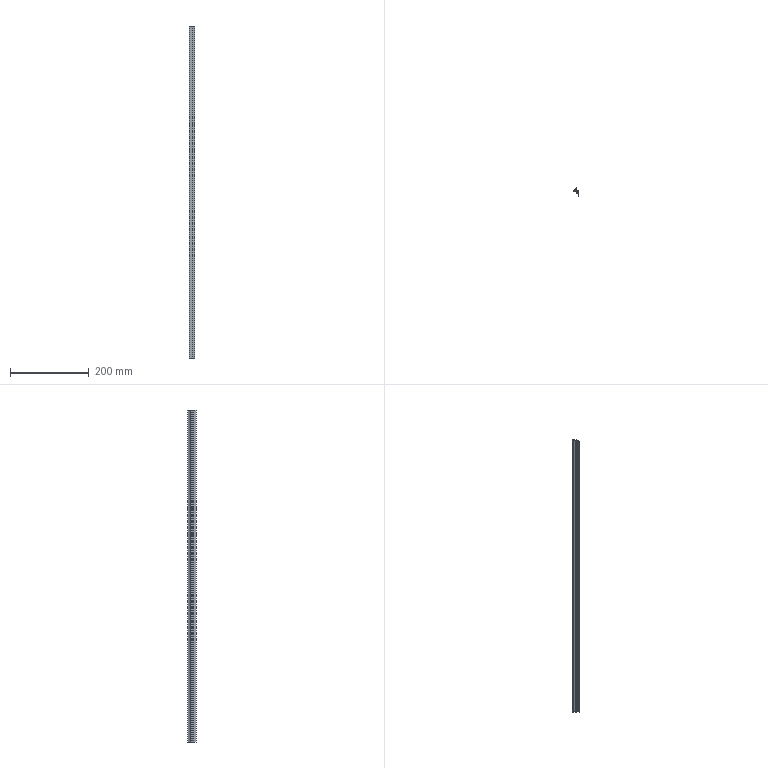Part | SolidWorks | features BaseBody 1, ICE 1, MoveFace 1 | 1 solid | 27 faces | box 14 x 20.3 x 842 mm | volume 42871 mm3 | plane 20 | cylinder 7 | commonest cylinder face diameters 0.387 x2 0.8 x2 0.4 x1 20 x1 22 x1
STEP:
#1=CARTESIAN_POINT('',(-5.304,-0.625,200.));
#2=VERTEX_POINT('',#1);
#3=CARTESIAN_POINT('',(-5.449,-0.8125,200.));
#4=VERTEX_POINT('',#3);
#5=CARTESIAN_POINT('',(-5.255,-0.8125,200.));
#6=DIRECTION('',(0.,0.,1.));
#7=DIRECTION('',(-1.,0.,0.));
#8=AXIS2_PLACEMENT_3D('',#5,#6,#7);
#9=CIRCLE('',#8,0.1937);
#10=EDGE_CURVE('',#2,#4,#9,.T.);
#11=ORIENTED_EDGE('',*,*,#10,.T.);
#12=CARTESIAN_POINT('',(-5.449,-0.8125,-642.));
#13=VERTEX_POINT('',#12);
#14=CARTESIAN_POINT('',(-5.449,-0.8125,230.));
#15=DIRECTION('',(0.,0.,-1.));
#16=VECTOR('',#15,1000.);
#17=LINE('',#14,#16);
#18=EDGE_CURVE('',#4,#13,#17,.T.);
#19=ORIENTED_EDGE('',*,*,#18,.T.);
#20=CARTESIAN_POINT('',(-5.304,-0.625,-642.));
#21=VERTEX_POINT('',#20);
#22=CARTESIAN_POINT('',(-5.255,-0.8125,-642.));
#23=DIRECTION('',(0.,0.,-1.));
#24=DIRECTION('',(1.,0.,0.));
#25=AXIS2_PLACEMENT_3D('',#22,#23,#24);
#26=CIRCLE('',#25,0.1937);
#27=EDGE_CURVE('',#13,#21,#26,.T.);
#28=ORIENTED_EDGE('',*,*,#27,.T.);
#29=CARTESIAN_POINT('',(-5.304,-0.625,230.));
#30=DIRECTION('',(0.,0.,-1.));
#31=VECTOR('',#30,1000.);
#32=LINE('',#29,#31);
#33=EDGE_CURVE('',#2,#21,#32,.T.);
#34=ORIENTED_EDGE('',*,*,#33,.F.);
#35=EDGE_LOOP('',(#11,#19,#28,#34));
#36=FACE_OUTER_BOUND('',#35,.T.);
#37=CARTESIAN_POINT('',(-5.255,-0.8125,230.));
#38=DIRECTION('',(0.,0.,-1.));
#39=DIRECTION('',(-1.,0.,0.));
#40=AXIS2_PLACEMENT_3D('',#37,#38,#39);
#41=CYLINDRICAL_SURFACE('',#40,0.1937);
#42=ADVANCED_FACE('',(#36),#41,.F.);
#43=CARTESIAN_POINT('',(5.,-1.,-642.));
#44=VERTEX_POINT('',#43);
#45=CARTESIAN_POINT('',(5.,-14.3,-642.));
#46=VERTEX_POINT('',#45);
#47=CARTESIAN_POINT('',(5.,29.623,-642.));
#48=DIRECTION('',(0.,-1.,0.));
#49=VECTOR('',#48,1000.);
#50=LINE('',#47,#49);
#51=EDGE_CURVE('',#44,#46,#50,.T.);
#52=ORIENTED_EDGE('',*,*,#51,.F.);
#53=CARTESIAN_POINT('',(5.,-1.,200.));
#54=VERTEX_POINT('',#53);
#55=CARTESIAN_POINT('',(5.,-1.,230.));
#56=DIRECTION('',(0.,0.,-1.));
#57=VECTOR('',#56,1000.);
#58=LINE('',#55,#57);
#59=EDGE_CURVE('',#54,#44,#58,.T.);
#60=ORIENTED_EDGE('',*,*,#59,.F.);
#61=CARTESIAN_POINT('',(5.,-14.3,200.));
#62=VERTEX_POINT('',#61);
#63=CARTESIAN_POINT('',(5.,-14.3,200.));
#64=DIRECTION('',(0.,1.,0.));
#65=VECTOR('',#64,1000.);
#66=LINE('',#63,#65);
#67=EDGE_CURVE('',#62,#54,#66,.T.);
#68=ORIENTED_EDGE('',*,*,#67,.F.);
#69=CARTESIAN_POINT('',(5.,-14.3,230.));
#70=DIRECTION('',(0.,0.,1.));
#71=VECTOR('',#70,1000.);
#72=LINE('',#69,#71);
#73=EDGE_CURVE('',#46,#62,#72,.T.);
#74=ORIENTED_EDGE('',*,*,#73,.F.);
#75=EDGE_LOOP('',(#52,#60,#68,#74));
#76=FACE_OUTER_BOUND('',#75,.T.);
#77=CARTESIAN_POINT('',(5.,-14.3,230.));
#78=DIRECTION('',(-1.,0.,0.));
#79=DIRECTION('',(0.,0.,1.));
#80=AXIS2_PLACEMENT_3D('',#77,#78,#79);
#81=PLANE('',#80);
#82=ADVANCED_FACE('',(#76),#81,.F.);
#83=CARTESIAN_POINT('',(-9.,-2.,-642.));
#84=VERTEX_POINT('',#83);
#85=CARTESIAN_POINT('',(-9.,-2.,200.));
#86=VERTEX_POINT('',#85);
#87=CARTESIAN_POINT('',(-9.,-2.,230.));
#88=DIRECTION('',(0.,0.,1.));
#89=VECTOR('',#88,1000.);
#90=LINE('',#87,#89);
#91=EDGE_CURVE('',#84,#86,#90,.T.);
#92=ORIENTED_EDGE('',*,*,#91,.F.);
#93=CARTESIAN_POINT('',(0.9,-2.,-642.));
#94=VERTEX_POINT('',#93);
#95=CARTESIAN_POINT('',(5.,-2.,-642.));
#96=DIRECTION('',(-1.,0.,0.));
#97=VECTOR('',#96,1000.);
#98=LINE('',#95,#97);
#99=EDGE_CURVE('',#94,#84,#98,.T.);
#100=ORIENTED_EDGE('',*,*,#99,.F.);
#101=CARTESIAN_POINT('',(0.9,-2.,200.));
#102=VERTEX_POINT('',#101);
#103=CARTESIAN_POINT('',(0.9,-2.,230.));
#104=DIRECTION('',(0.,0.,-1.));
#105=VECTOR('',#104,1000.);
#106=LINE('',#103,#105);
#107=EDGE_CURVE('',#102,#94,#106,.T.);
#108=ORIENTED_EDGE('',*,*,#107,.F.);
#109=CARTESIAN_POINT('',(5.,-2.,200.));
#110=DIRECTION('',(1.,0.,0.));
#111=VECTOR('',#110,1000.);
#112=LINE('',#109,#111);
#113=EDGE_CURVE('',#86,#102,#112,.T.);
#114=ORIENTED_EDGE('',*,*,#113,.F.);
#115=EDGE_LOOP('',(#92,#100,#108,#114));
#116=FACE_OUTER_BOUND('',#115,.T.);
#117=CARTESIAN_POINT('',(-9.,-2.,230.));
#118=DIRECTION('',(0.,1.,0.));
#119=DIRECTION('',(0.,0.,1.));
#120=AXIS2_PLACEMENT_3D('',#117,#118,#119);
#121=PLANE('',#120);
#122=ADVANCED_FACE('',(#116),#121,.F.);
#123=CARTESIAN_POINT('',(4.,-6.,200.));
#124=VERTEX_POINT('',#123);
#125=CARTESIAN_POINT('',(4.,-3.,200.));
#126=VERTEX_POINT('',#125);
#127=CARTESIAN_POINT('',(4.,29.623,200.));
#128=DIRECTION('',(0.,1.,0.));
#129=VECTOR('',#128,1000.);
#130=LINE('',#127,#129);
#131=EDGE_CURVE('',#124,#126,#130,.T.);
#132=ORIENTED_EDGE('',*,*,#131,.F.);
#133=CARTESIAN_POINT('',(1.,-6.,200.));
#134=VERTEX_POINT('',#133);
#135=CARTESIAN_POINT('',(5.,-6.,200.));
#136=DIRECTION('',(1.,0.,0.));
#137=VECTOR('',#136,1000.);
#138=LINE('',#135,#137);
#139=EDGE_CURVE('',#134,#124,#138,.T.);
#140=ORIENTED_EDGE('',*,*,#139,.F.);
#141=CARTESIAN_POINT('',(1.,-6.7,200.));
#142=VERTEX_POINT('',#141);
#143=CARTESIAN_POINT('',(1.,-6.,200.));
#144=DIRECTION('',(0.,-1.,0.));
#145=VECTOR('',#144,1000.);
#146=LINE('',#143,#145);
#147=EDGE_CURVE('',#134,#142,#146,.T.);
#148=ORIENTED_EDGE('',*,*,#147,.T.);
#149=CARTESIAN_POINT('',(-1.7,-6.7,200.));
#150=VERTEX_POINT('',#149);
#151=CARTESIAN_POINT('',(5.,-6.7,200.));
#152=DIRECTION('',(1.,0.,0.));
#153=VECTOR('',#152,1000.);
#154=LINE('',#151,#153);
#155=EDGE_CURVE('',#150,#142,#154,.T.);
#156=ORIENTED_EDGE('',*,*,#155,.F.);
#157=CARTESIAN_POINT('',(-1.7,-7.7,200.));
#158=VERTEX_POINT('',#157);
#159=CARTESIAN_POINT('',(-1.7,-6.7,200.));
#160=DIRECTION('',(0.,-1.,0.));
#161=VECTOR('',#160,1000.);
#162=LINE('',#159,#161);
#163=EDGE_CURVE('',#150,#158,#162,.T.);
#164=ORIENTED_EDGE('',*,*,#163,.T.);
#165=CARTESIAN_POINT('',(4.,-7.7,200.));
#166=VERTEX_POINT('',#165);
#167=CARTESIAN_POINT('',(5.,-7.7,200.));
#168=DIRECTION('',(-1.,0.,0.));
#169=VECTOR('',#168,1000.);
#170=LINE('',#167,#169);
#171=EDGE_CURVE('',#166,#158,#170,.T.);
#172=ORIENTED_EDGE('',*,*,#171,.F.);
#173=CARTESIAN_POINT('',(4.,-14.3,200.));
#174=VERTEX_POINT('',#173);
#175=CARTESIAN_POINT('',(4.,29.623,200.));
#176=DIRECTION('',(0.,1.,0.));
#177=VECTOR('',#176,1000.);
#178=LINE('',#175,#177);
#179=EDGE_CURVE('',#174,#166,#178,.T.);
#180=ORIENTED_EDGE('',*,*,#179,.F.);
#181=CARTESIAN_POINT('',(5.,-14.3,200.));
#182=DIRECTION('',(-1.,0.,0.));
#183=VECTOR('',#182,1000.);
#184=LINE('',#181,#183);
#185=EDGE_CURVE('',#62,#174,#184,.T.);
#186=ORIENTED_EDGE('',*,*,#185,.F.);
#187=ORIENTED_EDGE('',*,*,#67,.T.);
#188=CARTESIAN_POINT('',(-5.207,-1.,200.));
#189=VERTEX_POINT('',#188);
#190=CARTESIAN_POINT('',(5.,-1.,200.));
#191=DIRECTION('',(1.,0.,0.));
#192=VECTOR('',#191,1000.);
#193=LINE('',#190,#192);
#194=EDGE_CURVE('',#189,#54,#193,.T.);
#195=ORIENTED_EDGE('',*,*,#194,.F.);
#196=CARTESIAN_POINT('',(-5.255,-0.8125,200.));
#197=DIRECTION('',(0.,0.,1.));
#198=DIRECTION('',(-1.,0.,0.));
#199=AXIS2_PLACEMENT_3D('',#196,#197,#198);
#200=CIRCLE('',#199,0.1937);
#201=EDGE_CURVE('',#4,#189,#200,.T.);
#202=ORIENTED_EDGE('',*,*,#201,.F.);
#203=ORIENTED_EDGE('',*,*,#10,.F.);
#204=CARTESIAN_POINT('',(-1.368,3.063,200.));
#205=VERTEX_POINT('',#204);
#206=CARTESIAN_POINT('',(-10.628,9.,200.));
#207=DIRECTION('',(0.,0.,1.));
#208=DIRECTION('',(-1.,0.,0.));
#209=AXIS2_PLACEMENT_3D('',#206,#207,#208);
#210=CIRCLE('',#209,11.);
#211=EDGE_CURVE('',#2,#205,#210,.T.);
#212=ORIENTED_EDGE('',*,*,#211,.T.);
#213=CARTESIAN_POINT('',(-1.,2.955,200.));
#214=VERTEX_POINT('',#213);
#215=CARTESIAN_POINT('',(-1.2,2.955,200.));
#216=DIRECTION('',(0.,0.,1.));
#217=DIRECTION('',(-1.,0.,0.));
#218=AXIS2_PLACEMENT_3D('',#215,#216,#217);
#219=CIRCLE('',#218,0.2);
#220=EDGE_CURVE('',#214,#205,#219,.T.);
#221=ORIENTED_EDGE('',*,*,#220,.F.);
#222=CARTESIAN_POINT('',(-1.,1.5,200.));
#223=VERTEX_POINT('',#222);
#224=CARTESIAN_POINT('',(-1.,2.955,200.));
#225=DIRECTION('',(0.,1.,0.));
#226=VECTOR('',#225,1000.);
#227=LINE('',#224,#226);
#228=EDGE_CURVE('',#223,#214,#227,.T.);
#229=ORIENTED_EDGE('',*,*,#228,.F.);
#230=CARTESIAN_POINT('',(0.,1.5,200.));
#231=VERTEX_POINT('',#230);
#232=CARTESIAN_POINT('',(-1.,1.5,200.));
#233=DIRECTION('',(-1.,0.,0.));
#234=VECTOR('',#233,1000.);
#235=LINE('',#232,#234);
#236=EDGE_CURVE('',#231,#223,#235,.T.);
#237=ORIENTED_EDGE('',*,*,#236,.F.);
#238=CARTESIAN_POINT('',(0.,6.,200.));
#239=VERTEX_POINT('',#238);
#240=CARTESIAN_POINT('',(0.,1.5,200.));
#241=DIRECTION('',(0.,-1.,0.));
#242=VECTOR('',#241,1000.);
#243=LINE('',#240,#242);
#244=EDGE_CURVE('',#239,#231,#243,.T.);
#245=ORIENTED_EDGE('',*,*,#244,.F.);
#246=CARTESIAN_POINT('',(-0.8,6.,200.));
#247=VERTEX_POINT('',#246);
#248=CARTESIAN_POINT('',(0.,6.,200.));
#249=DIRECTION('',(1.,0.,0.));
#250=VECTOR('',#249,1000.);
#251=LINE('',#248,#250);
#252=EDGE_CURVE('',#247,#239,#251,.T.);
#253=ORIENTED_EDGE('',*,*,#252,.F.);
#254=CARTESIAN_POINT('',(-1.178,5.731,200.));
#255=VERTEX_POINT('',#254);
#256=CARTESIAN_POINT('',(-0.8,5.6,200.));
#257=DIRECTION('',(0.,0.,1.));
#258=DIRECTION('',(-1.,0.,0.));
#259=AXIS2_PLACEMENT_3D('',#256,#257,#258);
#260=CIRCLE('',#259,0.4);
#261=EDGE_CURVE('',#247,#255,#260,.T.);
#262=ORIENTED_EDGE('',*,*,#261,.T.);
#263=CARTESIAN_POINT('',(-8.678,-0.8077,200.));
#264=VERTEX_POINT('',#263);
#265=CARTESIAN_POINT('',(-10.628,9.,200.));
#266=DIRECTION('',(0.,0.,1.));
#267=DIRECTION('',(-1.,0.,0.));
#268=AXIS2_PLACEMENT_3D('',#265,#266,#267);
#269=CIRCLE('',#268,10.);
#270=EDGE_CURVE('',#264,#255,#269,.T.);
#271=ORIENTED_EDGE('',*,*,#270,.F.);
#272=CARTESIAN_POINT('',(-9.,-1.2,200.));
#273=VERTEX_POINT('',#272);
#274=CARTESIAN_POINT('',(-8.6,-1.2,200.));
#275=DIRECTION('',(0.,0.,1.));
#276=DIRECTION('',(-1.,0.,0.));
#277=AXIS2_PLACEMENT_3D('',#274,#275,#276);
#278=CIRCLE('',#277,0.4);
#279=EDGE_CURVE('',#264,#273,#278,.T.);
#280=ORIENTED_EDGE('',*,*,#279,.T.);
#281=CARTESIAN_POINT('',(-9.,8.,200.));
#282=DIRECTION('',(0.,-1.,0.));
#283=VECTOR('',#282,1000.);
#284=LINE('',#281,#283);
#285=EDGE_CURVE('',#273,#86,#284,.T.);
#286=ORIENTED_EDGE('',*,*,#285,.T.);
#287=ORIENTED_EDGE('',*,*,#113,.T.);
#288=CARTESIAN_POINT('',(0.9,-3.,200.));
#289=VERTEX_POINT('',#288);
#290=CARTESIAN_POINT('',(0.9,29.623,200.));
#291=DIRECTION('',(0.,1.,0.));
#292=VECTOR('',#291,1000.);
#293=LINE('',#290,#292);
#294=EDGE_CURVE('',#289,#102,#293,.T.);
#295=ORIENTED_EDGE('',*,*,#294,.F.);
#296=CARTESIAN_POINT('',(5.,-3.,200.));
#297=DIRECTION('',(-1.,0.,0.));
#298=VECTOR('',#297,1000.);
#299=LINE('',#296,#298);
#300=EDGE_CURVE('',#126,#289,#299,.T.);
#301=ORIENTED_EDGE('',*,*,#300,.F.);
#302=EDGE_LOOP('',(#132,#140,#148,#156,#164,#172,#180,#186,#187,#195,#202,#203,#212,#221,#229,#237,#245,#253,#262,#271,#280,#286,#287,#295,#301));
#303=FACE_OUTER_BOUND('',#302,.T.);
#304=CARTESIAN_POINT('',(5.,29.623,200.));
#305=DIRECTION('',(0.,0.,-1.));
#306=DIRECTION('',(-1.,0.,0.));
#307=AXIS2_PLACEMENT_3D('',#304,#305,#306);
#308=PLANE('',#307);
#309=ADVANCED_FACE('',(#303),#308,.F.);
#310=ORIENTED_EDGE('',*,*,#185,.T.);
#311=CARTESIAN_POINT('',(4.,-14.3,-642.));
#312=VERTEX_POINT('',#311);
#313=CARTESIAN_POINT('',(4.,-14.3,230.));
#314=DIRECTION('',(0.,0.,1.));
#315=VECTOR('',#314,1000.);
#316=LINE('',#313,#315);
#317=EDGE_CURVE('',#312,#174,#316,.T.);
#318=ORIENTED_EDGE('',*,*,#317,.F.);
#319=CARTESIAN_POINT('',(5.,-14.3,-642.));
#320=DIRECTION('',(-1.,0.,0.));
#321=VECTOR('',#320,1000.);
#322=LINE('',#319,#321);
#323=EDGE_CURVE('',#46,#312,#322,.T.);
#324=ORIENTED_EDGE('',*,*,#323,.F.);
#325=ORIENTED_EDGE('',*,*,#73,.T.);
#326=EDGE_LOOP('',(#310,#318,#324,#325));
#327=FACE_OUTER_BOUND('',#326,.T.);
#328=CARTESIAN_POINT('',(4.,-14.3,230.));
#329=DIRECTION('',(0.,1.,0.));
#330=DIRECTION('',(0.,0.,1.));
#331=AXIS2_PLACEMENT_3D('',#328,#329,#330);
#332=PLANE('',#331);
#333=ADVANCED_FACE('',(#327),#332,.F.);
#334=ORIENTED_EDGE('',*,*,#51,.T.);
#335=ORIENTED_EDGE('',*,*,#323,.T.);
#336=CARTESIAN_POINT('',(4.,-7.7,-642.));
#337=VERTEX_POINT('',#336);
#338=CARTESIAN_POINT('',(4.,-7.7,-642.));
#339=DIRECTION('',(0.,-1.,0.));
#340=VECTOR('',#339,1000.);
#341=LINE('',#338,#340);
#342=EDGE_CURVE('',#337,#312,#341,.T.);
#343=ORIENTED_EDGE('',*,*,#342,.F.);
#344=CARTESIAN_POINT('',(-1.7,-7.7,-642.));
#345=VERTEX_POINT('',#344);
#346=CARTESIAN_POINT('',(-1.7,-7.7,-642.));
#347=DIRECTION('',(1.,0.,0.));
#348=VECTOR('',#347,1000.);
#349=LINE('',#346,#348);
#350=EDGE_CURVE('',#345,#337,#349,.T.);
#351=ORIENTED_EDGE('',*,*,#350,.F.);
#352=CARTESIAN_POINT('',(-1.7,-6.7,-642.));
#353=VERTEX_POINT('',#352);
#354=CARTESIAN_POINT('',(-1.7,29.623,-642.));
#355=DIRECTION('',(0.,1.,0.));
#356=VECTOR('',#355,1000.);
#357=LINE('',#354,#356);
#358=EDGE_CURVE('',#345,#353,#357,.T.);
#359=ORIENTED_EDGE('',*,*,#358,.T.);
#360=CARTESIAN_POINT('',(1.,-6.7,-642.));
#361=VERTEX_POINT('',#360);
#362=CARTESIAN_POINT('',(1.,-6.7,-642.));
#363=DIRECTION('',(-1.,0.,0.));
#364=VECTOR('',#363,1000.);
#365=LINE('',#362,#364);
#366=EDGE_CURVE('',#361,#353,#365,.T.);
#367=ORIENTED_EDGE('',*,*,#366,.F.);
#368=CARTESIAN_POINT('',(1.,-6.,-642.));
#369=VERTEX_POINT('',#368);
#370=CARTESIAN_POINT('',(1.,29.623,-642.));
#371=DIRECTION('',(0.,1.,0.));
#372=VECTOR('',#371,1000.);
#373=LINE('',#370,#372);
#374=EDGE_CURVE('',#361,#369,#373,.T.);
#375=ORIENTED_EDGE('',*,*,#374,.T.);
#376=CARTESIAN_POINT('',(4.,-6.,-642.));
#377=VERTEX_POINT('',#376);
#378=CARTESIAN_POINT('',(4.,-6.,-642.));
#379=DIRECTION('',(-1.,0.,0.));
#380=VECTOR('',#379,1000.);
#381=LINE('',#378,#380);
#382=EDGE_CURVE('',#377,#369,#381,.T.);
#383=ORIENTED_EDGE('',*,*,#382,.F.);
#384=CARTESIAN_POINT('',(4.,-3.,-642.));
#385=VERTEX_POINT('',#384);
#386=CARTESIAN_POINT('',(4.,-3.,-642.));
#387=DIRECTION('',(0.,-1.,0.));
#388=VECTOR('',#387,1000.);
#389=LINE('',#386,#388);
#390=EDGE_CURVE('',#385,#377,#389,.T.);
#391=ORIENTED_EDGE('',*,*,#390,.F.);
#392=CARTESIAN_POINT('',(0.9,-3.,-642.));
#393=VERTEX_POINT('',#392);
#394=CARTESIAN_POINT('',(0.9,-3.,-642.));
#395=DIRECTION('',(1.,0.,0.));
#396=VECTOR('',#395,1000.);
#397=LINE('',#394,#396);
#398=EDGE_CURVE('',#393,#385,#397,.T.);
#399=ORIENTED_EDGE('',*,*,#398,.F.);
#400=CARTESIAN_POINT('',(0.9,-2.,-642.));
#401=DIRECTION('',(0.,-1.,0.));
#402=VECTOR('',#401,1000.);
#403=LINE('',#400,#402);
#404=EDGE_CURVE('',#94,#393,#403,.T.);
#405=ORIENTED_EDGE('',*,*,#404,.F.);
#406=ORIENTED_EDGE('',*,*,#99,.T.);
#407=CARTESIAN_POINT('',(-9.,-1.2,-642.));
#408=VERTEX_POINT('',#407);
#409=CARTESIAN_POINT('',(-9.,-1.2,-642.));
#410=DIRECTION('',(0.,-1.,0.));
#411=VECTOR('',#410,1000.);
#412=LINE('',#409,#411);
#413=EDGE_CURVE('',#408,#84,#412,.T.);
#414=ORIENTED_EDGE('',*,*,#413,.F.);
#415=CARTESIAN_POINT('',(-8.678,-0.8077,-642.));
#416=VERTEX_POINT('',#415);
#417=CARTESIAN_POINT('',(-8.6,-1.2,-642.));
#418=DIRECTION('',(0.,0.,-1.));
#419=DIRECTION('',(1.,0.,0.));
#420=AXIS2_PLACEMENT_3D('',#417,#418,#419);
#421=CIRCLE('',#420,0.4);
#422=EDGE_CURVE('',#408,#416,#421,.T.);
#423=ORIENTED_EDGE('',*,*,#422,.T.);
#424=CARTESIAN_POINT('',(-1.178,5.731,-642.));
#425=VERTEX_POINT('',#424);
#426=CARTESIAN_POINT('',(-10.628,9.,-642.));
#427=DIRECTION('',(0.,0.,-1.));
#428=DIRECTION('',(1.,0.,0.));
#429=AXIS2_PLACEMENT_3D('',#426,#427,#428);
#430=CIRCLE('',#429,10.);
#431=EDGE_CURVE('',#425,#416,#430,.T.);
#432=ORIENTED_EDGE('',*,*,#431,.F.);
#433=CARTESIAN_POINT('',(-0.8,6.,-642.));
#434=VERTEX_POINT('',#433);
#435=CARTESIAN_POINT('',(-0.8,5.6,-642.));
#436=DIRECTION('',(0.,0.,-1.));
#437=DIRECTION('',(1.,0.,0.));
#438=AXIS2_PLACEMENT_3D('',#435,#436,#437);
#439=CIRCLE('',#438,0.4);
#440=EDGE_CURVE('',#425,#434,#439,.T.);
#441=ORIENTED_EDGE('',*,*,#440,.T.);
#442=CARTESIAN_POINT('',(0.,6.,-642.));
#443=VERTEX_POINT('',#442);
#444=CARTESIAN_POINT('',(0.,6.,-642.));
#445=DIRECTION('',(-1.,0.,0.));
#446=VECTOR('',#445,1000.);
#447=LINE('',#444,#446);
#448=EDGE_CURVE('',#443,#434,#447,.T.);
#449=ORIENTED_EDGE('',*,*,#448,.F.);
#450=CARTESIAN_POINT('',(0.,1.5,-642.));
#451=VERTEX_POINT('',#450);
#452=CARTESIAN_POINT('',(0.,1.5,-642.));
#453=DIRECTION('',(0.,1.,0.));
#454=VECTOR('',#453,1000.);
#455=LINE('',#452,#454);
#456=EDGE_CURVE('',#451,#443,#455,.T.);
#457=ORIENTED_EDGE('',*,*,#456,.F.);
#458=CARTESIAN_POINT('',(-1.,1.5,-642.));
#459=VERTEX_POINT('',#458);
#460=CARTESIAN_POINT('',(-1.,1.5,-642.));
#461=DIRECTION('',(1.,0.,0.));
#462=VECTOR('',#461,1000.);
#463=LINE('',#460,#462);
#464=EDGE_CURVE('',#459,#451,#463,.T.);
#465=ORIENTED_EDGE('',*,*,#464,.F.);
#466=CARTESIAN_POINT('',(-1.,2.955,-642.));
#467=VERTEX_POINT('',#466);
#468=CARTESIAN_POINT('',(-1.,2.955,-642.));
#469=DIRECTION('',(0.,-1.,0.));
#470=VECTOR('',#469,1000.);
#471=LINE('',#468,#470);
#472=EDGE_CURVE('',#467,#459,#471,.T.);
#473=ORIENTED_EDGE('',*,*,#472,.F.);
#474=CARTESIAN_POINT('',(-1.368,3.063,-642.));
#475=VERTEX_POINT('',#474);
#476=CARTESIAN_POINT('',(-1.2,2.955,-642.));
#477=DIRECTION('',(0.,0.,-1.));
#478=DIRECTION('',(1.,0.,0.));
#479=AXIS2_PLACEMENT_3D('',#476,#477,#478);
#480=CIRCLE('',#479,0.2);
#481=EDGE_CURVE('',#475,#467,#480,.T.);
#482=ORIENTED_EDGE('',*,*,#481,.F.);
#483=CARTESIAN_POINT('',(-10.628,9.,-642.));
#484=DIRECTION('',(0.,0.,-1.));
#485=DIRECTION('',(1.,0.,0.));
#486=AXIS2_PLACEMENT_3D('',#483,#484,#485);
#487=CIRCLE('',#486,11.);
#488=EDGE_CURVE('',#475,#21,#487,.T.);
#489=ORIENTED_EDGE('',*,*,#488,.T.);
#490=ORIENTED_EDGE('',*,*,#27,.F.);
#491=CARTESIAN_POINT('',(-5.207,-1.,-642.));
#492=VERTEX_POINT('',#491);
#493=CARTESIAN_POINT('',(-5.255,-0.8125,-642.));
#494=DIRECTION('',(0.,0.,-1.));
#495=DIRECTION('',(1.,0.,0.));
#496=AXIS2_PLACEMENT_3D('',#493,#494,#495);
#497=CIRCLE('',#496,0.1937);
#498=EDGE_CURVE('',#492,#13,#497,.T.);
#499=ORIENTED_EDGE('',*,*,#498,.F.);
#500=CARTESIAN_POINT('',(5.,-1.,-642.));
#501=DIRECTION('',(-1.,0.,0.));
#502=VECTOR('',#501,1000.);
#503=LINE('',#500,#502);
#504=EDGE_CURVE('',#44,#492,#503,.T.);
#505=ORIENTED_EDGE('',*,*,#504,.F.);
#506=EDGE_LOOP('',(#334,#335,#343,#351,#359,#367,#375,#383,#391,#399,#405,#406,#414,#423,#432,#441,#449,#457,#465,#473,#482,#489,#490,#499,#505));
#507=FACE_OUTER_BOUND('',#506,.T.);
#508=CARTESIAN_POINT('',(5.,29.623,-642.));
#509=DIRECTION('',(0.,0.,1.));
#510=DIRECTION('',(1.,0.,0.));
#511=AXIS2_PLACEMENT_3D('',#508,#509,#510);
#512=PLANE('',#511);
#513=ADVANCED_FACE('',(#507),#512,.F.);
#514=ORIENTED_EDGE('',*,*,#59,.T.);
#515=ORIENTED_EDGE('',*,*,#504,.T.);
#516=CARTESIAN_POINT('',(-5.207,-1.,230.));
#517=DIRECTION('',(0.,0.,-1.));
#518=VECTOR('',#517,1000.);
#519=LINE('',#516,#518);
#520=EDGE_CURVE('',#189,#492,#519,.T.);
#521=ORIENTED_EDGE('',*,*,#520,.F.);
#522=ORIENTED_EDGE('',*,*,#194,.T.);
#523=EDGE_LOOP('',(#514,#515,#521,#522));
#524=FACE_OUTER_BOUND('',#523,.T.);
#525=CARTESIAN_POINT('',(5.,-1.,230.));
#526=DIRECTION('',(0.,-1.,0.));
#527=DIRECTION('',(0.,0.,-1.));
#528=AXIS2_PLACEMENT_3D('',#525,#526,#527);
#529=PLANE('',#528);
#530=ADVANCED_FACE('',(#524),#529,.F.);
#531=CARTESIAN_POINT('',(-9.,-1.2,230.));
#532=DIRECTION('',(0.,0.,1.));
#533=VECTOR('',#532,1000.);
#534=LINE('',#531,#533);
#535=EDGE_CURVE('',#408,#273,#534,.T.);
#536=ORIENTED_EDGE('',*,*,#535,.F.);
#537=ORIENTED_EDGE('',*,*,#413,.T.);
#538=ORIENTED_EDGE('',*,*,#91,.T.);
#539=ORIENTED_EDGE('',*,*,#285,.F.);
#540=EDGE_LOOP('',(#536,#537,#538,#539));
#541=FACE_OUTER_BOUND('',#540,.T.);
#542=CARTESIAN_POINT('',(-9.,-1.2,230.));
#543=DIRECTION('',(1.,0.,0.));
#544=DIRECTION('',(0.,0.,-1.));
#545=AXIS2_PLACEMENT_3D('',#542,#543,#544);
#546=PLANE('',#545);
#547=ADVANCED_FACE('',(#541),#546,.F.);
#548=ORIENTED_EDGE('',*,*,#294,.T.);
#549=ORIENTED_EDGE('',*,*,#107,.T.);
#550=ORIENTED_EDGE('',*,*,#404,.T.);
#551=CARTESIAN_POINT('',(0.9,-3.,230.));
#552=DIRECTION('',(0.,0.,-1.));
#553=VECTOR('',#552,1000.);
#554=LINE('',#551,#553);
#555=EDGE_CURVE('',#289,#393,#554,.T.);
#556=ORIENTED_EDGE('',*,*,#555,.F.);
#557=EDGE_LOOP('',(#548,#549,#550,#556));
#558=FACE_OUTER_BOUND('',#557,.T.);
#559=CARTESIAN_POINT('',(0.9,-2.,230.));
#560=DIRECTION('',(1.,0.,0.));
#561=DIRECTION('',(0.,0.,-1.));
#562=AXIS2_PLACEMENT_3D('',#559,#560,#561);
#563=PLANE('',#562);
#564=ADVANCED_FACE('',(#558),#563,.F.);
#565=ORIENTED_EDGE('',*,*,#300,.T.);
#566=ORIENTED_EDGE('',*,*,#555,.T.);
#567=ORIENTED_EDGE('',*,*,#398,.T.);
#568=CARTESIAN_POINT('',(4.,-3.,230.));
#569=DIRECTION('',(0.,0.,-1.));
#570=VECTOR('',#569,1000.);
#571=LINE('',#568,#570);
#572=EDGE_CURVE('',#126,#385,#571,.T.);
#573=ORIENTED_EDGE('',*,*,#572,.F.);
#574=EDGE_LOOP('',(#565,#566,#567,#573));
#575=FACE_OUTER_BOUND('',#574,.T.);
#576=CARTESIAN_POINT('',(0.9,-3.,230.));
#577=DIRECTION('',(0.,1.,0.));
#578=DIRECTION('',(0.,0.,1.));
#579=AXIS2_PLACEMENT_3D('',#576,#577,#578);
#580=PLANE('',#579);
#581=ADVANCED_FACE('',(#575),#580,.F.);
#582=ORIENTED_EDGE('',*,*,#131,.T.);
#583=ORIENTED_EDGE('',*,*,#572,.T.);
#584=ORIENTED_EDGE('',*,*,#390,.T.);
#585=CARTESIAN_POINT('',(4.,-6.,230.));
#586=DIRECTION('',(0.,0.,-1.));
#587=VECTOR('',#586,1000.);
#588=LINE('',#585,#587);
#589=EDGE_CURVE('',#124,#377,#588,.T.);
#590=ORIENTED_EDGE('',*,*,#589,.F.);
#591=EDGE_LOOP('',(#582,#583,#584,#590));
#592=FACE_OUTER_BOUND('',#591,.T.);
#593=CARTESIAN_POINT('',(4.,-3.,230.));
#594=DIRECTION('',(1.,0.,0.));
#595=DIRECTION('',(0.,0.,-1.));
#596=AXIS2_PLACEMENT_3D('',#593,#594,#595);
#597=PLANE('',#596);
#598=ADVANCED_FACE('',(#592),#597,.F.);
#599=ORIENTED_EDGE('',*,*,#139,.T.);
#600=ORIENTED_EDGE('',*,*,#589,.T.);
#601=ORIENTED_EDGE('',*,*,#382,.T.);
#602=CARTESIAN_POINT('',(1.,-6.,230.));
#603=DIRECTION('',(0.,0.,-1.));
#604=VECTOR('',#603,1000.);
#605=LINE('',#602,#604);
#606=EDGE_CURVE('',#134,#369,#605,.T.);
#607=ORIENTED_EDGE('',*,*,#606,.F.);
#608=EDGE_LOOP('',(#599,#600,#601,#607));
#609=FACE_OUTER_BOUND('',#608,.T.);
#610=CARTESIAN_POINT('',(4.,-6.,230.));
#611=DIRECTION('',(0.,-1.,0.));
#612=DIRECTION('',(0.,0.,-1.));
#613=AXIS2_PLACEMENT_3D('',#610,#611,#612);
#614=PLANE('',#613);
#615=ADVANCED_FACE('',(#609),#614,.F.);
#616=ORIENTED_EDGE('',*,*,#155,.T.);
#617=CARTESIAN_POINT('',(1.,-6.7,230.));
#618=DIRECTION('',(0.,0.,1.));
#619=VECTOR('',#618,1000.);
#620=LINE('',#617,#619);
#621=EDGE_CURVE('',#361,#142,#620,.T.);
#622=ORIENTED_EDGE('',*,*,#621,.F.);
#623=ORIENTED_EDGE('',*,*,#366,.T.);
#624=CARTESIAN_POINT('',(-1.7,-6.7,230.));
#625=DIRECTION('',(0.,0.,-1.));
#626=VECTOR('',#625,1000.);
#627=LINE('',#624,#626);
#628=EDGE_CURVE('',#150,#353,#627,.T.);
#629=ORIENTED_EDGE('',*,*,#628,.F.);
#630=EDGE_LOOP('',(#616,#622,#623,#629));
#631=FACE_OUTER_BOUND('',#630,.T.);
#632=CARTESIAN_POINT('',(1.,-6.7,230.));
#633=DIRECTION('',(0.,-1.,0.));
#634=DIRECTION('',(0.,0.,-1.));
#635=AXIS2_PLACEMENT_3D('',#632,#633,#634);
#636=PLANE('',#635);
#637=ADVANCED_FACE('',(#631),#636,.F.);
#638=ORIENTED_EDGE('',*,*,#171,.T.);
#639=CARTESIAN_POINT('',(-1.7,-7.7,230.));
#640=DIRECTION('',(0.,0.,1.));
#641=VECTOR('',#640,1000.);
#642=LINE('',#639,#641);
#643=EDGE_CURVE('',#345,#158,#642,.T.);
#644=ORIENTED_EDGE('',*,*,#643,.F.);
#645=ORIENTED_EDGE('',*,*,#350,.T.);
#646=CARTESIAN_POINT('',(4.,-7.7,230.));
#647=DIRECTION('',(0.,0.,-1.));
#648=VECTOR('',#647,1000.);
#649=LINE('',#646,#648);
#650=EDGE_CURVE('',#166,#337,#649,.T.);
#651=ORIENTED_EDGE('',*,*,#650,.F.);
#652=EDGE_LOOP('',(#638,#644,#645,#651));
#653=FACE_OUTER_BOUND('',#652,.T.);
#654=CARTESIAN_POINT('',(-1.7,-7.7,230.));
#655=DIRECTION('',(0.,1.,0.));
#656=DIRECTION('',(0.,0.,1.));
#657=AXIS2_PLACEMENT_3D('',#654,#655,#656);
#658=PLANE('',#657);
#659=ADVANCED_FACE('',(#653),#658,.F.);
#660=ORIENTED_EDGE('',*,*,#179,.T.);
#661=ORIENTED_EDGE('',*,*,#650,.T.);
#662=ORIENTED_EDGE('',*,*,#342,.T.);
#663=ORIENTED_EDGE('',*,*,#317,.T.);
#664=EDGE_LOOP('',(#660,#661,#662,#663));
#665=FACE_OUTER_BOUND('',#664,.T.);
#666=CARTESIAN_POINT('',(4.,-7.7,230.));
#667=DIRECTION('',(1.,0.,0.));
#668=DIRECTION('',(0.,0.,-1.));
#669=AXIS2_PLACEMENT_3D('',#666,#667,#668);
#670=PLANE('',#669);
#671=ADVANCED_FACE('',(#665),#670,.F.);
#672=ORIENTED_EDGE('',*,*,#18,.F.);
#673=ORIENTED_EDGE('',*,*,#201,.T.);
#674=ORIENTED_EDGE('',*,*,#520,.T.);
#675=ORIENTED_EDGE('',*,*,#498,.T.);
#676=EDGE_LOOP('',(#672,#673,#674,#675));
#677=FACE_OUTER_BOUND('',#676,.T.);
#678=CARTESIAN_POINT('',(-5.255,-0.8125,230.));
#679=DIRECTION('',(0.,0.,-1.));
#680=DIRECTION('',(-1.,0.,0.));
#681=AXIS2_PLACEMENT_3D('',#678,#679,#680);
#682=CYLINDRICAL_SURFACE('',#681,0.1937);
#683=ADVANCED_FACE('',(#677),#682,.F.);
#684=CARTESIAN_POINT('',(-1.,2.955,230.));
#685=DIRECTION('',(0.,0.,1.));
#686=VECTOR('',#685,1000.);
#687=LINE('',#684,#686);
#688=EDGE_CURVE('',#467,#214,#687,.T.);
#689=ORIENTED_EDGE('',*,*,#688,.F.);
#690=ORIENTED_EDGE('',*,*,#472,.T.);
#691=CARTESIAN_POINT('',(-1.,1.5,230.));
#692=DIRECTION('',(0.,0.,-1.));
#693=VECTOR('',#692,1000.);
#694=LINE('',#691,#693);
#695=EDGE_CURVE('',#223,#459,#694,.T.);
#696=ORIENTED_EDGE('',*,*,#695,.F.);
#697=ORIENTED_EDGE('',*,*,#228,.T.);
#698=EDGE_LOOP('',(#689,#690,#696,#697));
#699=FACE_OUTER_BOUND('',#698,.T.);
#700=CARTESIAN_POINT('',(-1.,2.955,230.));
#701=DIRECTION('',(1.,0.,0.));
#702=DIRECTION('',(0.,0.,-1.));
#703=AXIS2_PLACEMENT_3D('',#700,#701,#702);
#704=PLANE('',#703);
#705=ADVANCED_FACE('',(#699),#704,.F.);
#706=ORIENTED_EDGE('',*,*,#488,.F.);
#707=CARTESIAN_POINT('',(-1.368,3.063,230.));
#708=DIRECTION('',(0.,0.,1.));
#709=VECTOR('',#708,1000.);
#710=LINE('',#707,#709);
#711=EDGE_CURVE('',#475,#205,#710,.T.);
#712=ORIENTED_EDGE('',*,*,#711,.T.);
#713=ORIENTED_EDGE('',*,*,#211,.F.);
#714=ORIENTED_EDGE('',*,*,#33,.T.);
#715=EDGE_LOOP('',(#706,#712,#713,#714));
#716=FACE_OUTER_BOUND('',#715,.T.);
#717=CARTESIAN_POINT('',(-10.628,9.,230.));
#718=DIRECTION('',(0.,0.,-1.));
#719=DIRECTION('',(-1.,0.,0.));
#720=AXIS2_PLACEMENT_3D('',#717,#718,#719);
#721=CYLINDRICAL_SURFACE('',#720,11.);
#722=ADVANCED_FACE('',(#716),#721,.T.);
#723=CARTESIAN_POINT('',(-1.178,5.731,230.));
#724=DIRECTION('',(0.,0.,1.));
#725=VECTOR('',#724,1000.);
#726=LINE('',#723,#725);
#727=EDGE_CURVE('',#425,#255,#726,.T.);
#728=ORIENTED_EDGE('',*,*,#727,.F.);
#729=ORIENTED_EDGE('',*,*,#431,.T.);
#730=CARTESIAN_POINT('',(-8.678,-0.8077,230.));
#731=DIRECTION('',(0.,0.,-1.));
#732=VECTOR('',#731,1000.);
#733=LINE('',#730,#732);
#734=EDGE_CURVE('',#264,#416,#733,.T.);
#735=ORIENTED_EDGE('',*,*,#734,.F.);
#736=ORIENTED_EDGE('',*,*,#270,.T.);
#737=EDGE_LOOP('',(#728,#729,#735,#736));
#738=FACE_OUTER_BOUND('',#737,.T.);
#739=CARTESIAN_POINT('',(-10.628,9.,230.));
#740=DIRECTION('',(0.,0.,-1.));
#741=DIRECTION('',(-1.,0.,0.));
#742=AXIS2_PLACEMENT_3D('',#739,#740,#741);
#743=CYLINDRICAL_SURFACE('',#742,10.);
#744=ADVANCED_FACE('',(#738),#743,.F.);
#745=CARTESIAN_POINT('',(0.,1.5,230.));
#746=DIRECTION('',(0.,0.,1.));
#747=VECTOR('',#746,1000.);
#748=LINE('',#745,#747);
#749=EDGE_CURVE('',#451,#231,#748,.T.);
#750=ORIENTED_EDGE('',*,*,#749,.F.);
#751=ORIENTED_EDGE('',*,*,#456,.T.);
#752=CARTESIAN_POINT('',(0.,6.,230.));
#753=DIRECTION('',(0.,0.,-1.));
#754=VECTOR('',#753,1000.);
#755=LINE('',#752,#754);
#756=EDGE_CURVE('',#239,#443,#755,.T.);
#757=ORIENTED_EDGE('',*,*,#756,.F.);
#758=ORIENTED_EDGE('',*,*,#244,.T.);
#759=EDGE_LOOP('',(#750,#751,#757,#758));
#760=FACE_OUTER_BOUND('',#759,.T.);
#761=CARTESIAN_POINT('',(0.,1.5,230.));
#762=DIRECTION('',(-1.,0.,0.));
#763=DIRECTION('',(0.,0.,1.));
#764=AXIS2_PLACEMENT_3D('',#761,#762,#763);
#765=PLANE('',#764);
#766=ADVANCED_FACE('',(#760),#765,.F.);
#767=ORIENTED_EDGE('',*,*,#422,.F.);
#768=ORIENTED_EDGE('',*,*,#535,.T.);
#769=ORIENTED_EDGE('',*,*,#279,.F.);
#770=ORIENTED_EDGE('',*,*,#734,.T.);
#771=EDGE_LOOP('',(#767,#768,#769,#770));
#772=FACE_OUTER_BOUND('',#771,.T.);
#773=CARTESIAN_POINT('',(-8.6,-1.2,230.));
#774=DIRECTION('',(0.,0.,-1.));
#775=DIRECTION('',(-1.,0.,0.));
#776=AXIS2_PLACEMENT_3D('',#773,#774,#775);
#777=CYLINDRICAL_SURFACE('',#776,0.4);
#778=ADVANCED_FACE('',(#772),#777,.T.);
#779=ORIENTED_EDGE('',*,*,#147,.F.);
#780=ORIENTED_EDGE('',*,*,#606,.T.);
#781=ORIENTED_EDGE('',*,*,#374,.F.);
#782=ORIENTED_EDGE('',*,*,#621,.T.);
#783=EDGE_LOOP('',(#779,#780,#781,#782));
#784=FACE_OUTER_BOUND('',#783,.T.);
#785=CARTESIAN_POINT('',(1.,-6.,230.));
#786=DIRECTION('',(1.,0.,0.));
#787=DIRECTION('',(0.,0.,-1.));
#788=AXIS2_PLACEMENT_3D('',#785,#786,#787);
#789=PLANE('',#788);
#790=ADVANCED_FACE('',(#784),#789,.F.);
#791=ORIENTED_EDGE('',*,*,#163,.F.);
#792=ORIENTED_EDGE('',*,*,#628,.T.);
#793=ORIENTED_EDGE('',*,*,#358,.F.);
#794=ORIENTED_EDGE('',*,*,#643,.T.);
#795=EDGE_LOOP('',(#791,#792,#793,#794));
#796=FACE_OUTER_BOUND('',#795,.T.);
#797=CARTESIAN_POINT('',(-1.7,-6.7,230.));
#798=DIRECTION('',(1.,0.,0.));
#799=DIRECTION('',(0.,0.,-1.));
#800=AXIS2_PLACEMENT_3D('',#797,#798,#799);
#801=PLANE('',#800);
#802=ADVANCED_FACE('',(#796),#801,.F.);
#803=ORIENTED_EDGE('',*,*,#711,.F.);
#804=ORIENTED_EDGE('',*,*,#481,.T.);
#805=ORIENTED_EDGE('',*,*,#688,.T.);
#806=ORIENTED_EDGE('',*,*,#220,.T.);
#807=EDGE_LOOP('',(#803,#804,#805,#806));
#808=FACE_OUTER_BOUND('',#807,.T.);
#809=CARTESIAN_POINT('',(-1.2,2.955,230.));
#810=DIRECTION('',(0.,0.,-1.));
#811=DIRECTION('',(-1.,0.,0.));
#812=AXIS2_PLACEMENT_3D('',#809,#810,#811);
#813=CYLINDRICAL_SURFACE('',#812,0.2);
#814=ADVANCED_FACE('',(#808),#813,.F.);
#815=ORIENTED_EDGE('',*,*,#695,.T.);
#816=ORIENTED_EDGE('',*,*,#464,.T.);
#817=ORIENTED_EDGE('',*,*,#749,.T.);
#818=ORIENTED_EDGE('',*,*,#236,.T.);
#819=EDGE_LOOP('',(#815,#816,#817,#818));
#820=FACE_OUTER_BOUND('',#819,.T.);
#821=CARTESIAN_POINT('',(-1.,1.5,230.));
#822=DIRECTION('',(0.,1.,0.));
#823=DIRECTION('',(0.,0.,1.));
#824=AXIS2_PLACEMENT_3D('',#821,#822,#823);
#825=PLANE('',#824);
#826=ADVANCED_FACE('',(#820),#825,.F.);
#827=ORIENTED_EDGE('',*,*,#440,.F.);
#828=ORIENTED_EDGE('',*,*,#727,.T.);
#829=ORIENTED_EDGE('',*,*,#261,.F.);
#830=CARTESIAN_POINT('',(-0.8,6.,230.));
#831=DIRECTION('',(0.,0.,-1.));
#832=VECTOR('',#831,1000.);
#833=LINE('',#830,#832);
#834=EDGE_CURVE('',#247,#434,#833,.T.);
#835=ORIENTED_EDGE('',*,*,#834,.T.);
#836=EDGE_LOOP('',(#827,#828,#829,#835));
#837=FACE_OUTER_BOUND('',#836,.T.);
#838=CARTESIAN_POINT('',(-0.8,5.6,230.));
#839=DIRECTION('',(0.,0.,-1.));
#840=DIRECTION('',(-1.,0.,0.));
#841=AXIS2_PLACEMENT_3D('',#838,#839,#840);
#842=CYLINDRICAL_SURFACE('',#841,0.4);
#843=ADVANCED_FACE('',(#837),#842,.T.);
#844=ORIENTED_EDGE('',*,*,#756,.T.);
#845=ORIENTED_EDGE('',*,*,#448,.T.);
#846=ORIENTED_EDGE('',*,*,#834,.F.);
#847=ORIENTED_EDGE('',*,*,#252,.T.);
#848=EDGE_LOOP('',(#844,#845,#846,#847));
#849=FACE_OUTER_BOUND('',#848,.T.);
#850=CARTESIAN_POINT('',(0.,6.,230.));
#851=DIRECTION('',(0.,-1.,0.));
#852=DIRECTION('',(0.,0.,-1.));
#853=AXIS2_PLACEMENT_3D('',#850,#851,#852);
#854=PLANE('',#853);
#855=ADVANCED_FACE('',(#849),#854,.F.);
#856=CLOSED_SHELL('',(#42,#82,#122,#309,#333,#513,#530,#547,#564,#581,#598,#615,#637,#659,#671,#683,#705,#722,#744,#766,#778,#790,#802,#814,#826,#843,#855));
#857=MANIFOLD_SOLID_BREP('',#856);
#858=CARTESIAN_POINT('',(0.,0.,0.));
#859=DIRECTION('',(0.,0.,1.));
#860=DIRECTION('',(1.,0.,0.));
#861=AXIS2_PLACEMENT_3D('',#858,#859,#860);
#862=(LENGTH_UNIT()NAMED_UNIT(*)SI_UNIT(.MILLI.,.METRE.));
#863=UNCERTAINTY_MEASURE_WITH_UNIT(LENGTH_MEASURE(0.00001),#862,'','');
#864=(NAMED_UNIT(*)PLANE_ANGLE_UNIT()SI_UNIT($,.RADIAN.));
#865=(NAMED_UNIT(*)SI_UNIT($,.STERADIAN.)SOLID_ANGLE_UNIT());
#866=(GEOMETRIC_REPRESENTATION_CONTEXT(3)GLOBAL_UNCERTAINTY_ASSIGNED_CONTEXT((#863))GLOBAL_UNIT_ASSIGNED_CONTEXT((#862,#864,#865))REPRESENTATION_CONTEXT('',''));
#867=ADVANCED_BREP_SHAPE_REPRESENTATION('',(#857,#861),#866);